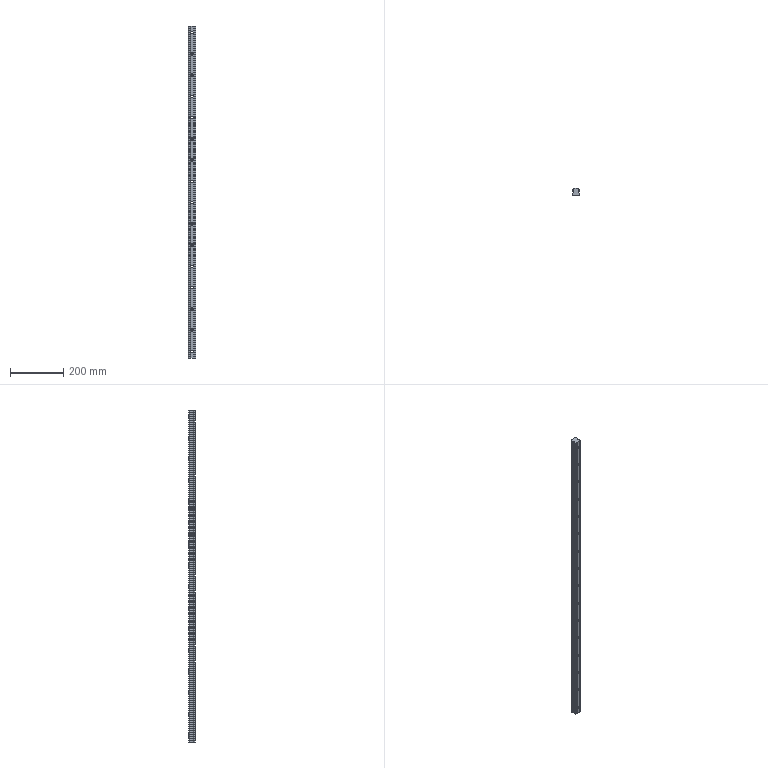Part | STEP file | linear guide HGR30HC-1250-25-25 | 1 solid | 132 faces | box 28 x 26 x 1250 mm | volume 722759 mm3 | cylinder 86 | plane 46 | commonest cylinder face diameters 9 x32 14 x32 1.2 x12 1.6 x6 5.66 x4